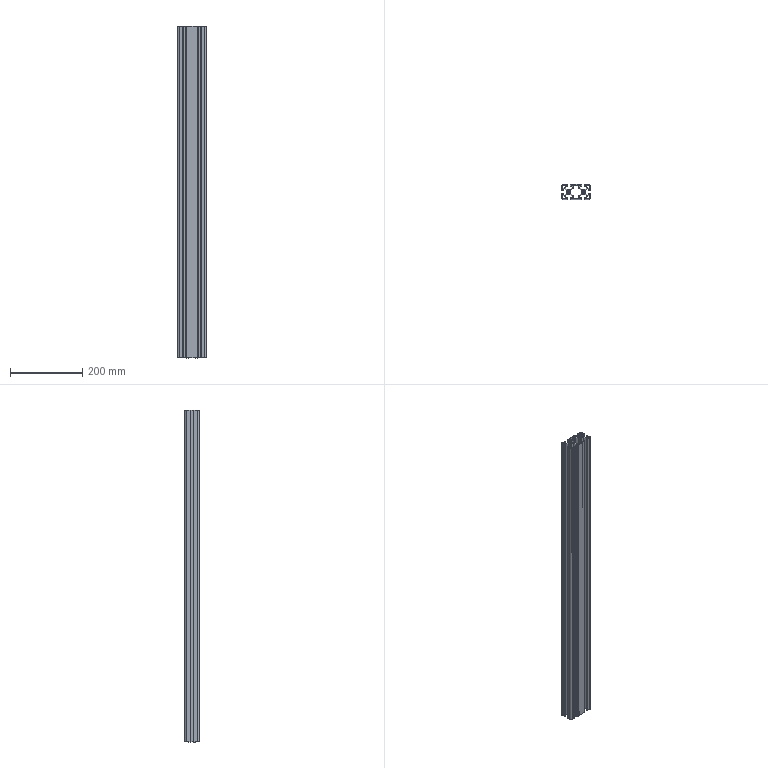Part | STEP file | LE-8-4080-S-OO_LE0313224113 | 1 solid | 286 faces | box 80 x 40 x 920 mm | volume 739877 mm3 | cylinder 144 | plane 142 | commonest cylinder face diameters 0.6 x48 2 x36 4 x28 0.4 x12 5 x4 6 x4